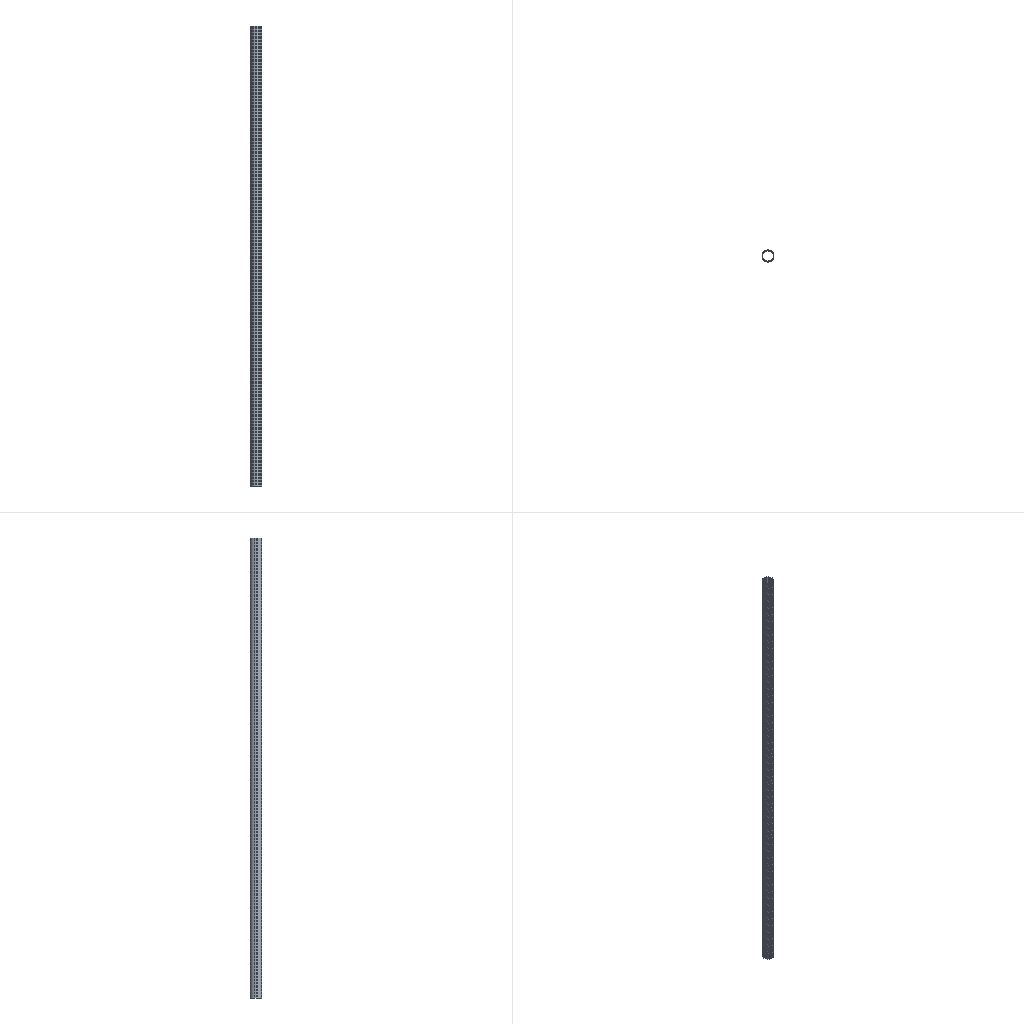Simulation study | ansys workbench
Set-up summary:
category,name,step,type,value,unit,region
solver,ansys_mapdl
solver,version,,,24.2
units,MPA,,stated
analysis,deck,,static,static
load_step,requested,,,1
analysis,nlgeom,,,False
mesh,nodes,,,57344
mesh,elements,,,11680
element_type,ANSYS 186 (type 1),,solid,3136
element_type,ANSYS 186 (type 2),,solid,2688
element_type,ANSYS 186 (type 3),,solid,3136
element_type,ANSYS 174 (type 4),,contact,56
element_type,ANSYS 170 (type 5),,target,56
element_type,ANSYS 174 (type 6),,contact,56
element_type,ANSYS 170 (type 7),,target,56
element_type,ANSYS 154 (type 8),,surface,2496
load,load commands in deck,,count,3
bc,support commands in deck,,count,1
named_set,_FIXEDSU,,component
material,1,,in results
material,2,,in results
material,3,,in results
check,setup vs results,,match,112 contact/target element(s) of the setup are not in the results: ZST-1/廷旭-23个(1)/有限元仿真/碳纤维管/碳纤维圆柱体_files/dp0/SYS/MECH/solve.out records that the solver deleted 112 by its trimming logic; 2496 surface effect element(s) are not in the reader's mesh and were not compared
Ansys APDL input file, long lists of numbers shortened:
/batch
/config,noeldb,1     ! force off writing results to database
*get,_wallstrt,active,,time,wall
! ANSYS input file written by Workbench version 2024 R2
! File used for geometry attach: C:\Users\USER_\Desktop\ç»æ.STEP
/title,wbnew--____ (A5)
! ****** Begin Custom Load Command Snippet ******
/COM, ACT Extensions:
/COM,     LSDYNA, 2024.2
/COM,/COM,     ANSYSMotion, 2024.2
/COM,
! ****** End   Custom Load Command Snippet ******
*DIM,_wb_ProjectScratch_dir,string,248
_wb_ProjectScratch_dir(1) = 'C:\Users\USER_\AppData\Local\Temp\WB_86130_155144_2\_ProjectScratch\Scr92A0\'
*DIM,_wb_SolverFiles_dir,string,248
_wb_SolverFiles_dir(1) = 'C:\Users\USER_\AppData\Local\Temp\WB_86130_155144_2\wbnew_files\dp0\SYS\MECH\'
*DIM,_wb_userfiles_dir,string,248
_wb_userfiles_dir(1) = 'C:\Users\USER_\AppData\Local\Temp\WB_86130_155144_2\wbnew_files\user_files\'
/com,--- Data in consistent NMM units. See Solving Units in the help system for more information.
/units,MPA
/nopr
/wb,file,start              !  signify a WB generated input file
/prep7
! Turn off shape checking because checks already performed inside WB mesher.
! See help system for more information.
SHPP,OFF,,NOWARN
/nolist
etcon,set             ! allow ANSYS to choose best KEYOP's for 180x elements, resets any applicable keyopt to MAPDL defaults
/com,*********** Nodes for the whole assembly ***********
nblock,3,,63078
(1i9,3e20.9e3)
    20065     1.145031694E+01     6.878590737E+00     2.040000000E+03
! (57343 more lines like these left out)
-1
/wb,elem,start            !  set before creation of elements
/com,*********** Elements for Body 1 '__1|__-__1' ***********
et,1,186
keyo,1,2,1          ! set full integration on SOLID186
eblock,19,solid,,3136
(19i9)
        1        1        1        1        0        0        0        0       20        0        1       56       57     3080     3081     1278     1277     4412     4413
! (6271 more lines like these left out)
-1
/com,*********** Elements for Body 2 '__2|__-__1' ***********
et,2,186
keyo,2,2,1          ! set full integration on SOLID186
eblock,19,solid,,2688
(19i9)
        2        2        2        2        0        0        0        0       20        0     3137    21155    23840    23839    21156    21165    23852    23851    21164
! (5375 more lines like these left out)
-1
/com,*********** Elements for Body 3 '__1|__-__1[2]' ***********
et,3,186
keyo,3,2,1          ! set full integration on SOLID186
eblock,19,solid,,3136
(19i9)
        3        3        3        3        0        0        0        0       20        0     5825    37336    37337    40360    40361    38558    38557    41692    41693
! (6271 more lines like these left out)
-1
/wb,elem,end               !  done creating elements
/com,*********** Send User Defined Coordinate System(s) ***********
csys,0
toffst,273.15,      ! Temperature offset from absolute zero
/com,*********** Set Reference Temperature ***********
tref,22.
/wb,mat,start              !  starting to send materials
/com,*********** Send Materials ***********
MP,EX,1,230000,	! tonne s^-2 mm^-1
MP,EY,1,23000,	! tonne s^-2 mm^-1
MP,EZ,1,23000,	! tonne s^-2 mm^-1
MP,PRXY,1,0.2,
! (32 more lines like these left out)
/wb,mat,end                !  done sending materials
!************************* Model Summary ********************
!é¶ä»¶1|å¸å°-æä¼¸1,	ç¢³çº¤ç»´ææ,	matid,	1
!é¶ä»¶2|å¸å°-æä¼¸1,	ç¢³çº¤ç»´ææ,	matid,	2
!é¶ä»¶1|å¸å°-æä¼¸1[2],	ç¢³çº¤ç»´ææ,	matid,	3
!************************* End Model Summary ********************
! get the diagonal of the bounding box. Needed later for other things
*get,_xmin,node,,mnloc,x
*get,_ymin,node,,mnloc,y
*get,_zmin,node,,mnloc,z
*get,_xmax,node,,mxloc,x
*get,_ymax,node,,mxloc,y
*get,_zmax,node,,mxloc,z
_ASMDIAG=(_xmax-_xmin)*(_xmax-_xmin)+(_ymax-_ymin)*(_ymax-_ymin)+(_zmax-_zmin)*(_zmax-_zmin)
_ASMDIAG=SQRT(_ASMDIAG)
/wb,contact,start          !  starting to send contact
/com,*********** Create Contact "½Ó´¥ÇøÓò" ***********
/com,            Real Constant Set For Above Contact Is 5 & 4
*set,tid,5
*set,cid,4
r,tid
r,cid
et,tid,170
et,cid,174
eblock,10,,,28
(15i9)
    25129        5        5        5        0     1277     1276     4411     4411     9785     9787     4411     9789
! (27 more lines like these left out)
-1
eblock,10,,,28
(15i9)
    25157        4        4        4        0     1277     1276     4411     4411     9785     9787     4411     9789
! (27 more lines like these left out)
-1
eblock,10,,,28
(15i9)
    25185        4        5        4        0    21166    21167    23853    23853    28478    28481    23853    28479
! (27 more lines like these left out)
-1
eblock,10,,,28
(15i9)
    25213        5        4        5        0    21166    21167    23853    23853    28478    28481    23853    28479
! (27 more lines like these left out)
-1
keyo,cid,8,2               ! auto create asymmetric contact (from Program Controlled setting)
keyo,cid,10,0              ! adjust contact stiffness each NR iteration (from Program Controlled setting)
keyo,cid,12,5              ! bonded always
keyo,cid,18,1              ! small sliding turned on by application
keyo,cid,2,0               ! augmented Lagrange (from Program Controlled setting)
keyo,cid,4,0               ! on Gauss point (from Program Controlled setting)
keyo,cid,9,1               ! ignore initial gaps/penetration
keyo,cid,7,0               ! No Prediction
rmod,tid,3,10.      ! FKN
rmod,tid,5,0.       ! ICONT
rmod,tid,6,0.       ! PINB
rmod,tid,10,0.      ! CNOF
rmod,tid,12,0.      ! FKT
rmod,tid,36,33      ! WB DSID
rmod,cid,3,10.      ! FKN
rmod,cid,5,0.       ! ICONT
rmod,cid,6,0.       ! PINB
rmod,cid,10,0.      ! CNOF
rmod,cid,12,0.      ! FKT
rmod,cid,36,33      ! WB DSID
/com,*********** Create Contact "½Ó´¥ÇøÓò 2" ***********
/com,            Real Constant Set For Above Contact Is 7 & 6
*set,tid,7
*set,cid,6
r,tid
r,cid
et,tid,170
et,cid,174
eblock,10,,,28
(15i9)
    25241        7        7        7        0    20108    20082    20109    20109    24971    24972    20109    25030
! (27 more lines like these left out)
-1
eblock,10,,,28
(15i9)
    25269        6        6        6        0    20108    20082    20109    20109    24971    24972    20109    25030
! (27 more lines like these left out)
-1
eblock,10,,,28
(15i9)
    25297        6        7        6        0    37323    37296    37322    37322    42982    42981    37322    43042
! (27 more lines like these left out)
-1
eblock,10,,,28
(15i9)
    25325        7        6        7        0    37323    37296    37322    37322    42982    42981    37322    43042
! (27 more lines like these left out)
-1
keyo,cid,8,2               ! auto create asymmetric contact (from Program Controlled setting)
keyo,cid,10,0              ! adjust contact stiffness each NR iteration (from Program Controlled setting)
keyo,cid,12,5              ! bonded always
keyo,cid,18,1              ! small sliding turned on by application
keyo,cid,2,0               ! augmented Lagrange (from Program Controlled setting)
keyo,cid,4,0               ! on Gauss point (from Program Controlled setting)
keyo,cid,9,1               ! ignore initial gaps/penetration
keyo,cid,7,0               ! No Prediction
rmod,tid,3,10.      ! FKN
rmod,tid,5,0.       ! ICONT
rmod,tid,6,0.       ! PINB
rmod,tid,10,0.      ! CNOF
rmod,tid,12,0.      ! FKT
rmod,tid,36,36      ! WB DSID
rmod,cid,3,10.      ! FKN
rmod,cid,5,0.       ! ICONT
rmod,cid,6,0.       ! PINB
rmod,cid,10,0.      ! CNOF
rmod,cid,12,0.      ! FKT
rmod,cid,36,36      ! WB DSID
nsel,all
esel,all
/wb,contact,end            !  done creating contacts
/golist
/wb,load,start             !  starting to send loads
/com,*********** Fixed Supports ***********
CMBLOCK,_FIXEDSU,NODE,    17576
(8i10)
        12        13        14        15        16        17        18        19
! (2196 more lines like these left out)
cmsel,s,_FIXEDSU
d,all,all
nsel,all
/com,*********** Define Force Using Surface Effect Elements ***********
local,12,0,0.,0.,0.,0.,0.,0.
csys,0
et,8,154
mat,8
eblock,10,,,2496
(15i9)
    25353        8        8        8       12    22517    22707    20076    20100    32703    24954    24952    25016
! (2495 more lines like these left out)
-1
esel,s,type,,8
keyop,8,2,1         ! Apply load in local coordinate system
keyop,8,7,1         ! Use original area so load is constant in large deformation
esel,all
/gst,on,on
fini
*get,_numnode,node,0,count
*get,_numelem,elem,0,count
*get, _MAXELEMNUM, elem, 0, NUM, MAX
*get, _MAXNODENUM, node, 0, NUM, MAX
*get, _MAXELEMTYPE, etyp, 0, NUM, MAX
*get, _MAXREALCONST, rcon, 0, NUM, MAX
/go
/wb,load,end               !  done creating loads
/com,--- Number of total nodes = %_numnode%
/com,--- Number of contact elements = 2720
/com,--- Number of spring elements = 0
/com,--- Number of bearing elements = 0
/com,--- Number of solid elements = 8960
/com,--- Number of condensed parts = 0
/com,--- Number of total elements = %_numelem%
*get,_wallbsol,active,,time,wall
/com,****************************************************************************
/com,*************************    SOLUTION       ********************************
/com,****************************************************************************
/solu
antype,0                   ! static analysis
_thickRatio=  0     ! Ratio of thick parts in the model
eqsl,sparse,,,,,1
cntr,print,1               ! print out contact info and also make no initial contact an error
cncheck,dmp		!	Enable program controlled contact splitting for distributed memory parallel run
dmpoption,emat,no             ! Don't combine emat file for DANSYS
dmpoption,esav,no             ! Don't combine esav file for DANSYS
nldiag,cont,iter           ! print out contact info each equilibrium iteration
rescontrol,,none                 ! Do not keep any restart files
/com,****************************************************
/com,******************* SOLVE FOR LS 1 OF 1 ****************
esel,s,type,,8
nsle
sfe,all,1,pres,1,0.
sfe,all,2,pres,1,0.173
sfe,all,3,pres,1,0.
nsel,all
esel,all
/nopr
/gopr
nsub,1,1,1
time,1.
outres,erase
outres,all,none
outres,nsol,all,
outres,rsol,all
outres,eangl,all
outres,etmp,all
outres,veng,all
outres,strs,all,
outres,epel,all,
outres,eppl,all,
outres,cont,all,
! *********** WB SOLVE COMMAND ***********
! check interactive state
*get,ANSINTER_,active,,int
*if,ANSINTER_,ne,0,then
/eof
*endif
solve
/com *************** Write FE CONNECTORS *********
CEWRITE,file,ce,,INTE
/com,****************************************************
/com,*************** FINISHED SOLVE FOR LS 1 *************
*get,_wallasol,active,,time,wall
/nopr
*get,_numnode,node,0,count
*get,_numelem,elem,0,count
*get, _MAXELEMNUM, elem, 0, NUM, MAX
*get, _MAXNODENUM, node, 0, NUM, MAX,,,INTERNAL
*get, _MAXELEMTYPE, etyp, 0, NUM, MAX
*get, _MAXREALCONST, rcon, 0, NUM, MAX
*get,_NSOLTHREADS,active,0,ntfs
*get,_NSOLPROCESSES,active,0,npfs
/gopr
/post1
xmlo,ENCODING,ISO-8859-1
xmlo,parm
/xml,parm,xml
fini
/gopr
*get,_walldone,active,,time,wall
_preptime=(_wallbsol-_wallstrt)*3600
_solvtime=(_wallasol-_wallbsol)*3600
_posttime=(_walldone-_wallasol)*3600
_totaltim=(_walldone-_wallstrt)*3600
*get,_dlbratio,active,0,solu,dlbr
*get,_combtime,active,0,solu,comb
*get,_ssmode,active,0,solu,ssmm
*get,_ndofs,active,0,solu,ndof
*get,_sol_end_time,active,0,set,time
*if,_sol_end_time,eq,1.,then
/fclean				!clean distributed files
*endif
/com,--- Total number of nodes = %_numnode%
/com,--- Total number of elements = %_numelem%
/com,--- Element load balance ratio = %_dlbratio%
/com,--- Time to combine distributed files = %_combtime%
/com,--- Sparse memory mode = %_ssmode%
/com,--- Number of DOF = %_ndofs%
/wb,file,end               ! done with WB generated input
Results summary:
result,analysis,,,static
result,last_loadstep,,,1
result,primary field,,,displacement
result,reaction total,1,FX,0.0,N
result,reaction total,1,FY,-10398.0,N
result,reaction total,1,FZ,-0.0,N
result,mass,,,0.000495,"NMM: mm, ton, N, s, mV, mA, degC"